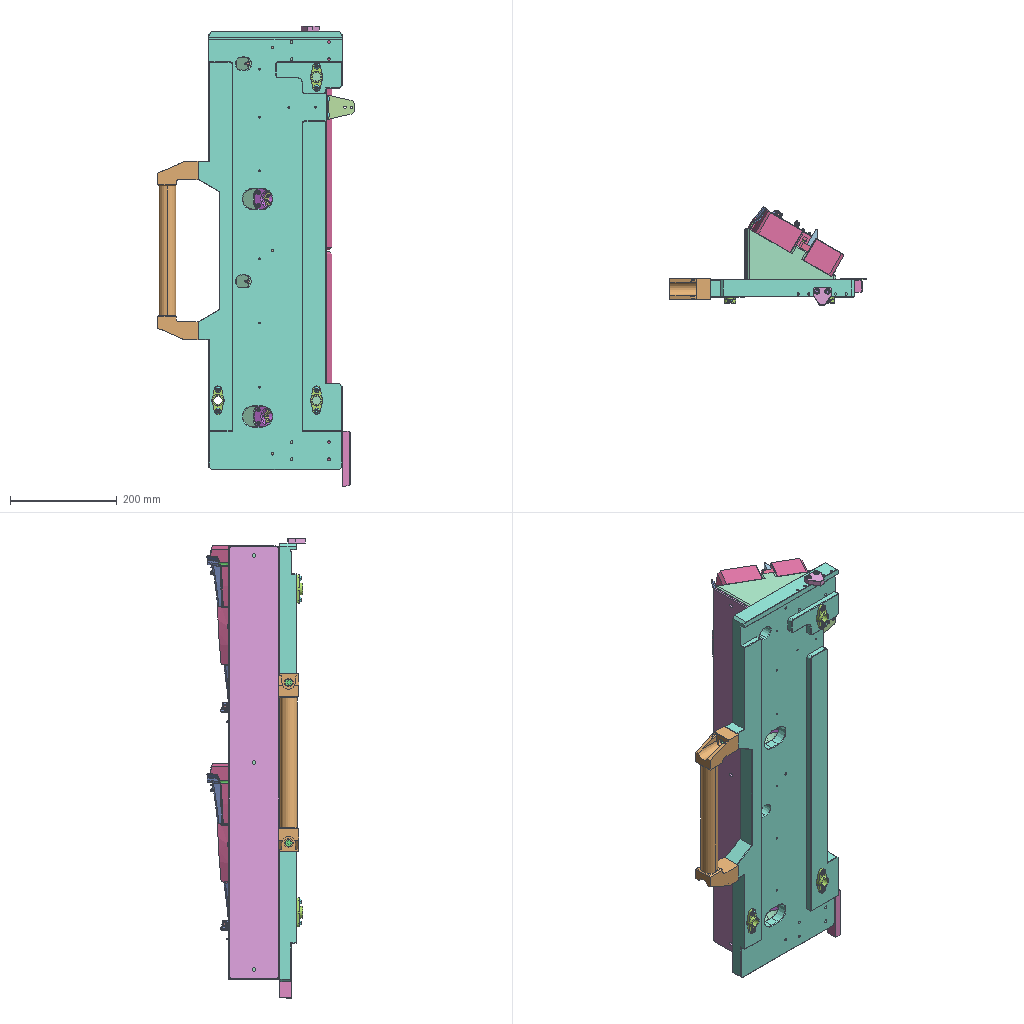Assembly | SolidWorks | 30 different items | 84 placed | box 367 x 184 x 861 mm
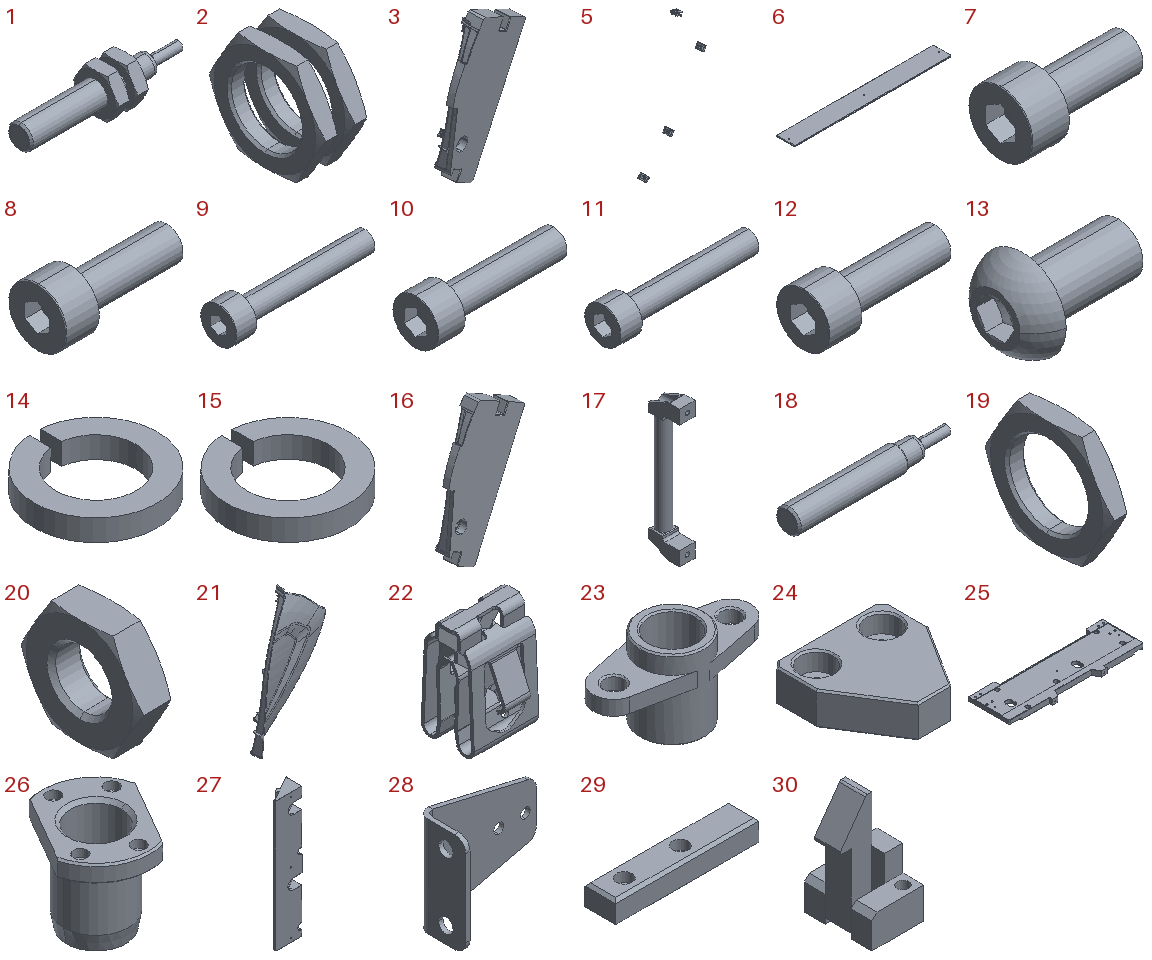Parts list (item | name | quantity | parent item | size | volume | features):
1 | (subassembly) | x2 | - | 52.05 x 15.011 x 13 mm | 2912 mm3 | features AEMSimFeature 1
2 | (subassembly) | x2 | - | 11 x 27.713 x 24 mm | 2123 mm3 | features AEMSimFeature 1
3 | (subassembly) | x2 | - | - | 2042090 mm3 | features AEMSimFeature 1
4 | (subassembly) | x2 | in 5 | - | - | features AEMSimFeature 1
5 | (subassembly) | x2 | in 3 | 133.256 x 34.357 x 254.473 mm | 678.705 mm3 | features AEMSimFeature 1
6 | - | x1 | - | 810 x 95 x 6 mm | 456909 mm3 | features Chamfer 1, Extrusion 1, Fillet 1, ICE 1
7 | - | x2 | - | 17 x 8.5 x 8.5 mm | 483.388 mm3 | features BlendCut 1, Cut 1, Fillet 1, LPattern 1, RevCut 1, Revolution 1
8 | - | x8 | - | 16 x 7 x 7 mm | 288.227 mm3 | features BlendCut 1, Cut 1, Fillet 1, LPattern 1, RevCut 1, Revolution 1
9 | - | x8 | - | 29 x 7 x 7 mm | 451.59 mm3 | features BlendCut 1, Cut 1, Fillet 1, LPattern 1, RevCut 1, Revolution 1
10 | - | x2 | - | 31 x 10 x 10 mm | 1111 mm3 | features BlendCut 1, Cut 1, Fillet 1, LPattern 1, RevCut 1, Revolution 1
11 | - | x3 | - | 41 x 10 x 10 mm | 1393 mm3 | features BlendCut 1, Cut 1, Fillet 1, LPattern 1, RevCut 1, Revolution 1
12 | - | x2 | - | 33 x 13 x 13 mm | 2189 mm3 | features BlendCut 1, Cut 1, Fillet 1, LPattern 1, RevCut 1, Revolution 1
13 | - | x8 | - | 15.3 x 10.5 x 10.5 mm | 508.665 mm3 | features RevCut 2, Revolution 2, Cut 1, LPattern 1, RefAxis 1
14 | - | x1 | - | 6.287 x 6.275 x 1.1 mm | 18.963 mm3 | features Extrusion 1
15 | - | x2 | - | 9.282 x 9.265 x 1.6 mm | 59.463 mm3 | features Extrusion 1
16 | - | x2 | in 3 | - | - | features ICE 56, Chamfer 17, 3DProfileFeature 16, FillRefSurface 11, OffsetRefSurface 6, Fillet 2, BaseBody 1, DeleteBody 1, ExtendRefSurface 1, Thicken 1, TrimRefSurface 1
17 | - | x1 | - | 38 x 75 x 334 mm | 331639 mm3 | features BaseBody 1
18 | - | x2 | in 1 | 52.05 x 8 x 8 mm | 2062 mm3 | features BaseBody 1
19 | - | x4 | in 2 | 4 x 27.713 x 24 mm | 1061 mm3 | features BaseBody 1
20 | - | x4 | in 1 | 4 x 15.011 x 13 mm | 425.34 mm3 | features BaseBody 1
21 | - | x2 | in 3 | 209.02 x 66.466 x 351.204 mm | 105260 mm3 | features BaseBody 1
22 | - | x8 | in 5 | 9.4 x 10.589 x 14.619 mm | 169.677 mm3 | features BaseBody 1
23 | - | x3 | - | 54 x 22 x 27 mm | 6993 mm3 | features ICE 3, 3DProfileFeature 1, Chamfer 1, Extrusion 1, HoleWzd 1
24 | - | x1 | - | 34 x 33 x 10 mm | 7759 mm3 | features Chamfer 2, 3DProfileFeature 1, Extrusion 1, HoleWzd 1, ICE 1
25 | - | x1 | - | 820.75 x 270 x 32.5 mm | 4272161 mm3 | features ICE 22, Chamfer 16, 3DProfileFeature 11, HoleWzd 11, Fillet 3, LPattern 2, Extrusion 1
26 | - | x2 | - | 61.725 x 64 x 55 mm | 43113 mm3 | features Chamfer 4, ICE 3, 3DProfileFeature 2, HoleWzd 2, CirPattern 1, Extrusion 1
27 | - | x1 | - | 165 x 98.335 x 810.75 mm | 6353061 mm3 | features Chamfer 11, ICE 11, 3DProfileFeature 4, HoleWzd 4, Fillet 2, LPattern 2, CirPattern 1, Extrusion 1
28 | - | x1 | - | 52 x 22 x 45 mm | 5057 mm3 | features ICE 3, Extrusion 1, Fillet 1
29 | - | x1 | - | 102 x 22 x 15 mm | 31316 mm3 | features Chamfer 2, 3DProfileFeature 1, Extrusion 1, HoleWzd 1
30 | - | x4 | - | 24 x 26 x 45 mm | 8320 mm3 | features ICE 4, Chamfer 1, Extrusion 1, Fillet 1
Mates (type | each side: item.copy, entity, surface, feature):
In the top assembly
Coincident | 16.1 face plane Cut-Extrude9 | 27.1 face plane Cut-Extrude1
Coincident | 16.1 face plane Boss-Extrude1 | 27.1 face plane Boss-Extrude1
Parallel | 16.1 face plane Boss-Extrude1 | 16.2 face plane Boss-Extrude1
Concentric | 16.1 face cylinder Cut-Extrude1 | 26.1 face cylinder Boss-Extrude1
Parallel | 16.1 face plane Boss-Extrude1 | 27.1 face plane Boss-Extrude1
DistanceDim | 30.1 face plane Boss-Extrude3 | 16.1 face plane Cut-Extrude16
DistanceDim | 30.2 face plane Boss-Extrude3 | 16.1 face plane Cut-Extrude16
DistanceDim | 30.2 face plane Boss-Extrude1 | 16.1 face plane Boss-Extrude1
Concentric | 23.1 face cylinder Boss-Extrude1 | 25.1 face cylinder LPattern3
Concentric | 23.2 face cylinder Boss-Extrude1 | 25.1 face cylinder Cut-Extrude7
Coincident | 25.1 face plane Boss-Extrude3 | 17.1 face plane Input1
Concentric | 25.1 face cylinder M8 Tapped Hole2 | 17.1 face cylinder Input1
Parallel | 25.1 face plane Boss-Extrude1 | 17.1 face plane Input1
Coincident | 25.1 face plane Cut-Extrude20 | 27.1 face plane Boss-Extrude1 | 2 times
Width | 25.1 face plane Cut-Extrude20 | 25.1 face plane Cut-Extrude20 | 27.1 face plane Boss-Extrude1 | 27.1 face plane Boss-Extrude1
Coincident | 8.1 face plane Boss-Revolve | 14.1 face plane Extrude1
Concentric | 8.1 face cylinder Boss-Revolve | 14.1 face cylinder Extrude1
Concentric | 8.1 face cylinder Boss-Revolve | 26.1 face cylinder CirPattern1
Coincident | 14.1 face plane Extrude1 | 26.1 face plane CirPattern1
Coincident | 30.1 face plane Boss-Extrude1 | 27.1 face plane Boss-Extrude2
DistanceDim | 30.1 face plane Boss-Extrude1 | 27.1 face plane Boss-Extrude1
Coincident | 30.2 face plane Boss-Extrude1 | 27.1 face plane Boss-Extrude2
Coincident | assembly face | 26.1 face plane Boss-Extrude1
Concentric | assembly face | 26.1 face cylinder M18x1.5 Tapped Hole1
Concentric | 26.1 face cylinder Boss-Extrude1 | 27.1 face cylinder Cut-Extrude3
Parallel | 26.1 face plane Cut-Extrude2 | 27.1 face plane Boss-Extrude1
Coincident | 26.1 face plane Boss-Extrude2 | 27.1 face plane Cut-Extrude6
Coincident | 27.1 face plane Cut-Extrude1 | 16.2 face plane Cut-Extrude9
Coincident | 27.1 face plane Cut-Extrude1 | 18.1 face plane Input1
Concentric | 27.1 face cylinder M8x1.0 Tapped Hole1 | 18.1 face cylinder Input1
Coincident | 23.2 face plane Boss-Extrude2 | 25.1 face plane Cut-Extrude29
Coincident | 23.1 face plane Boss-Extrude2 | 25.1 face plane Cut-Extrude29
Concentric | 24.1 face cylinder Hole size per socket head cap screw type1 | 25.1 face cylinder M5 Tapped Hole4 | 2 times
Coincident | 24.1 face plane Boss-Extrude1 | 25.1 face plane Boss-Extrude1
Concentric | 25.1 face cylinder Cut-Extrude30 | 23.3 face cylinder Boss-Extrude1
Concentric | 25.1 face cylinder M6 Tapped Hole4 | 23.3 face cylinder Hole size per socket head cap screw type1
Coincident | 25.1 face plane Cut-Extrude29 | 23.3 face plane Boss-Extrude2
Coincident | 25.1 face plane Boss-Extrude1 | 28.1 face plane Boss-Extrude1
Concentric | 25.1 face cylinder M6 Tapped Hole3 | 28.1 face cylinder Cut-Extrude1 | 2 times
Coincident | 25.1 face plane Boss-Extrude4 | 29.1 face plane Boss-Extrude1
Concentric | 25.1 face cylinder M6 Tapped Hole5 | 29.1 face cylinder Hole size per socket head cap screw type1 | 2 times
Parallel | 25.1 face plane Boss-Extrude1 | assembly plane | 2 times
Coincident | 16.1 face plane Boss-Extrude1 | 16.2 face plane Boss-Extrude1
Coincident | 23.1 face plane Hole size per socket head cap screw type1 | 13.1 face plane Revolve1
Concentric | 23.1 face cylinder Hole size per socket head cap screw type1 | 13.1 face cylinder Revolve1
Coincident | 27.1 face plane Cut-Extrude10 | 11.1 face plane Boss-Revolve
Concentric | 27.1 face cylinder Ø7.0 (7) Diameter Hole1 | 11.1 face cylinder Boss-Revolve
Coincident | 24.1 face plane Hole size per socket head cap screw type1 | 7.1 face plane Boss-Revolve
Concentric | 24.1 face cylinder Hole size per socket head cap screw type1 | 7.1 face cylinder Boss-Revolve
Coincident | 17.1 face plane Input1 | 12.1 face plane Boss-Revolve
Concentric | 17.1 face cylinder Input1 | 12.1 face cylinder Boss-Revolve
Coincident | 10.1 face plane Boss-Revolve | 15.1 face plane Extrude1
Concentric | 10.1 face cylinder Boss-Revolve | 15.1 face cylinder Extrude1
Coincident | 29.1 face plane Hole size per socket head cap screw type1 | 15.1 face plane Extrude1
Concentric | 29.1 face cylinder Hole size per socket head cap screw type1 | 10.1 face cylinder Boss-Revolve
Coincident | 28.1 face plane Boss-Extrude1 | 13.2 face plane Revolve1
Concentric | 25.1 face cylinder M6 Tapped Hole3 | 13.2 face cylinder Revolve1
Coincident | 30.1 face plane Boss-Extrude1 | 9.1 face plane Boss-Revolve
Concentric | 30.1 face cylinder Cut-Extrude1 | 9.1 face cylinder Boss-Revolve
Coincident | 27.1 face plane Boss-Extrude1 | 6.1 face plane Boss-Extrude1 | 2 times
Coincident | 25.1 face plane Boss-Extrude1 | 6.1 face plane Boss-Extrude1
In subassembly 3
DistanceDim | 3.1 vertex | 16.3 vertex
DistanceDim | 16.3 vertex | 3.1 vertex
Coincident | 3.1 face | 21.1 face plane Input2 | 3 times
In subassembly 5
Width | 5.1 face | 5.1 face | 22.1 face plane Input1 | 22.1 face plane Input1
Tangent | 5.1 face | 22.1 face plane Input1
Width | 5.1 face | 5.1 face | 22.2 face plane Input1 | 22.2 face plane Input1
Tangent | 5.1 face | 22.2 face plane Input1
Width | 5.1 face | 5.1 face | 22.3 face plane Input1 | 22.3 face plane Input1
Tangent | 5.1 face | 22.3 face plane Input1
Tangent | 5.1 face | 22.4 face plane Input1
Width | 5.1 face | 5.1 face | 22.4 face plane Input1 | 22.4 face plane Input1
In subassembly 1
Concentric | 18.2 face cylinder Input1 | 20.1 face cylinder Input1
Concentric | 18.2 face cylinder Input1 | 20.2 face cylinder Input1